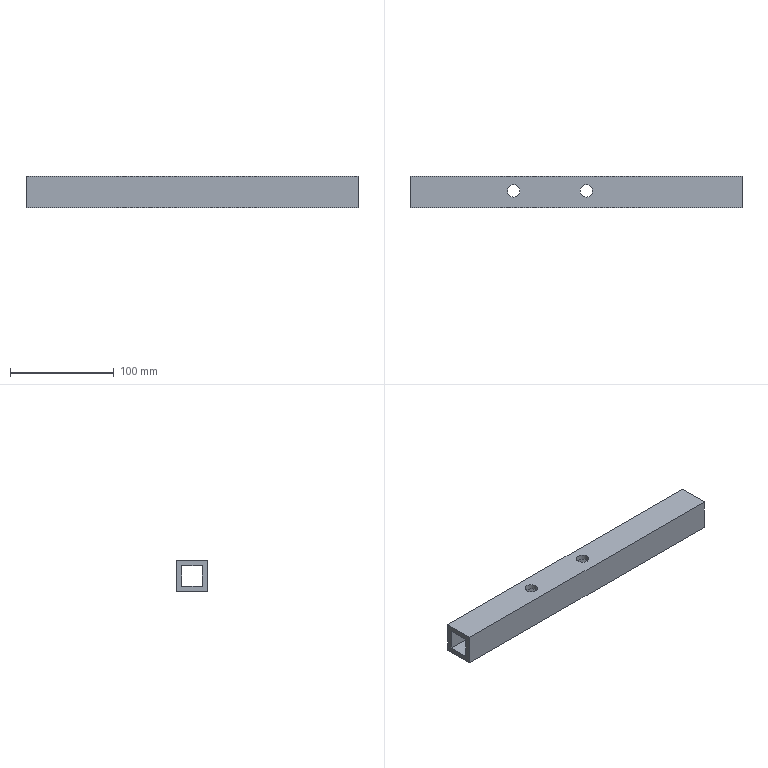Part | NX | features solid 2 | 1 solid | 14 faces | box 320 x 30 x 30 mm | volume 157738 mm3 | plane 10 | cylinder 4 | commonest cylinder face diameters 12 x4
STEP:
#1=CARTESIAN_POINT('',(65.,-206.,-122.));
#2=VERTEX_POINT('',#1);
#3=CARTESIAN_POINT('',(385.,-206.,-122.));
#4=VERTEX_POINT('',#3);
#5=CARTESIAN_POINT('',(132.005,-206.,-122.));
#6=DIRECTION('',(1.,0.,0.));
#7=VECTOR('',#6,1000.);
#8=LINE('',#5,#7);
#9=EDGE_CURVE('',#2,#4,#8,.T.);
#10=ORIENTED_EDGE('',*,*,#9,.T.);
#11=CARTESIAN_POINT('',(385.,-236.,-122.));
#12=VERTEX_POINT('',#11);
#13=CARTESIAN_POINT('',(385.,5.001,-122.));
#14=DIRECTION('',(0.,1.,0.));
#15=VECTOR('',#14,1000.);
#16=LINE('',#13,#15);
#17=EDGE_CURVE('',#12,#4,#16,.T.);
#18=ORIENTED_EDGE('',*,*,#17,.F.);
#19=CARTESIAN_POINT('',(65.,-236.,-122.));
#20=VERTEX_POINT('',#19);
#21=CARTESIAN_POINT('',(292.505,-236.,-122.));
#22=DIRECTION('',(1.,0.,0.));
#23=VECTOR('',#22,1000.);
#24=LINE('',#21,#23);
#25=EDGE_CURVE('',#20,#12,#24,.T.);
#26=ORIENTED_EDGE('',*,*,#25,.F.);
#27=CARTESIAN_POINT('',(65.,-206.,-122.));
#28=DIRECTION('',(0.,-1.,0.));
#29=VECTOR('',#28,1000.);
#30=LINE('',#27,#29);
#31=EDGE_CURVE('',#2,#20,#30,.T.);
#32=ORIENTED_EDGE('',*,*,#31,.F.);
#33=EDGE_LOOP('',(#10,#18,#26,#32));
#34=FACE_BOUND('',#33,.T.);
#35=CARTESIAN_POINT('',(165.,-226.,-122.));
#36=VERTEX_POINT('',#35);
#37=CARTESIAN_POINT('',(165.,-220.,-122.));
#38=DIRECTION('',(0.,0.,-1.));
#39=DIRECTION('',(0.,-1.,0.));
#40=AXIS2_PLACEMENT_3D('',#37,#38,#39);
#41=CIRCLE('',#40,6.);
#42=EDGE_CURVE('',#36,#36,#41,.T.);
#43=ORIENTED_EDGE('',*,*,#42,.F.);
#44=EDGE_LOOP('',(#43));
#45=FACE_BOUND('',#44,.T.);
#46=CARTESIAN_POINT('',(235.,-226.,-122.));
#47=VERTEX_POINT('',#46);
#48=CARTESIAN_POINT('',(235.,-220.,-122.));
#49=DIRECTION('',(0.,0.,1.));
#50=DIRECTION('',(0.,-1.,0.));
#51=AXIS2_PLACEMENT_3D('',#48,#49,#50);
#52=CIRCLE('',#51,6.);
#53=EDGE_CURVE('',#47,#47,#52,.T.);
#54=ORIENTED_EDGE('',*,*,#53,.T.);
#55=EDGE_LOOP('',(#54));
#56=FACE_BOUND('',#55,.T.);
#57=CARTESIAN_POINT('',(132.005,-206.5,-122.));
#58=DIRECTION('',(0.,0.,-1.));
#59=DIRECTION('',(0.,-1.,0.));
#60=AXIS2_PLACEMENT_3D('',#57,#58,#59);
#61=PLANE('',#60);
#62=ADVANCED_FACE('',(#34,#45,#56),#61,.T.);
#63=CARTESIAN_POINT('',(65.,-236.,-92.));
#64=VERTEX_POINT('',#63);
#65=CARTESIAN_POINT('',(385.,-236.,-92.));
#66=VERTEX_POINT('',#65);
#67=CARTESIAN_POINT('',(132.005,-236.,-92.));
#68=DIRECTION('',(1.,0.,0.));
#69=VECTOR('',#68,1000.);
#70=LINE('',#67,#69);
#71=EDGE_CURVE('',#64,#66,#70,.T.);
#72=ORIENTED_EDGE('',*,*,#71,.T.);
#73=CARTESIAN_POINT('',(385.,-206.,-92.));
#74=VERTEX_POINT('',#73);
#75=CARTESIAN_POINT('',(385.,5.001,-92.));
#76=DIRECTION('',(0.,-1.,0.));
#77=VECTOR('',#76,1000.);
#78=LINE('',#75,#77);
#79=EDGE_CURVE('',#74,#66,#78,.T.);
#80=ORIENTED_EDGE('',*,*,#79,.F.);
#81=CARTESIAN_POINT('',(65.,-206.,-92.));
#82=VERTEX_POINT('',#81);
#83=CARTESIAN_POINT('',(132.005,-206.,-92.));
#84=DIRECTION('',(1.,0.,0.));
#85=VECTOR('',#84,1000.);
#86=LINE('',#83,#85);
#87=EDGE_CURVE('',#82,#74,#86,.T.);
#88=ORIENTED_EDGE('',*,*,#87,.F.);
#89=CARTESIAN_POINT('',(65.,-236.5,-92.));
#90=DIRECTION('',(0.,1.,0.));
#91=VECTOR('',#90,1000.);
#92=LINE('',#89,#91);
#93=EDGE_CURVE('',#64,#82,#92,.T.);
#94=ORIENTED_EDGE('',*,*,#93,.F.);
#95=EDGE_LOOP('',(#72,#80,#88,#94));
#96=FACE_BOUND('',#95,.T.);
#97=CARTESIAN_POINT('',(165.,-226.,-92.));
#98=VERTEX_POINT('',#97);
#99=CARTESIAN_POINT('',(165.,-220.,-92.));
#100=DIRECTION('',(0.,0.,1.));
#101=DIRECTION('',(0.,-1.,0.));
#102=AXIS2_PLACEMENT_3D('',#99,#100,#101);
#103=CIRCLE('',#102,6.);
#104=EDGE_CURVE('',#98,#98,#103,.T.);
#105=ORIENTED_EDGE('',*,*,#104,.F.);
#106=EDGE_LOOP('',(#105));
#107=FACE_BOUND('',#106,.T.);
#108=CARTESIAN_POINT('',(235.,-226.,-92.));
#109=VERTEX_POINT('',#108);
#110=CARTESIAN_POINT('',(235.,-220.,-92.));
#111=DIRECTION('',(0.,0.,1.));
#112=DIRECTION('',(0.,-1.,0.));
#113=AXIS2_PLACEMENT_3D('',#110,#111,#112);
#114=CIRCLE('',#113,6.);
#115=EDGE_CURVE('',#109,#109,#114,.F.);
#116=ORIENTED_EDGE('',*,*,#115,.T.);
#117=EDGE_LOOP('',(#116));
#118=FACE_BOUND('',#117,.T.);
#119=CARTESIAN_POINT('',(132.005,-236.5,-92.));
#120=DIRECTION('',(0.,0.,1.));
#121=DIRECTION('',(0.,1.,0.));
#122=AXIS2_PLACEMENT_3D('',#119,#120,#121);
#123=PLANE('',#122);
#124=ADVANCED_FACE('',(#96,#107,#118),#123,.T.);
#125=CARTESIAN_POINT('',(65.,-211.,-117.));
#126=VERTEX_POINT('',#125);
#127=CARTESIAN_POINT('',(385.,-211.,-117.));
#128=VERTEX_POINT('',#127);
#129=CARTESIAN_POINT('',(132.005,-211.,-117.));
#130=DIRECTION('',(1.,0.,0.));
#131=VECTOR('',#130,1000.);
#132=LINE('',#129,#131);
#133=EDGE_CURVE('',#126,#128,#132,.T.);
#134=ORIENTED_EDGE('',*,*,#133,.F.);
#135=CARTESIAN_POINT('',(65.,-231.,-117.));
#136=VERTEX_POINT('',#135);
#137=CARTESIAN_POINT('',(65.,-206.5,-117.));
#138=DIRECTION('',(0.,-1.,0.));
#139=VECTOR('',#138,1000.);
#140=LINE('',#137,#139);
#141=EDGE_CURVE('',#126,#136,#140,.T.);
#142=ORIENTED_EDGE('',*,*,#141,.T.);
#143=CARTESIAN_POINT('',(385.,-231.,-117.));
#144=VERTEX_POINT('',#143);
#145=CARTESIAN_POINT('',(292.505,-231.,-117.));
#146=DIRECTION('',(1.,0.,0.));
#147=VECTOR('',#146,1000.);
#148=LINE('',#145,#147);
#149=EDGE_CURVE('',#136,#144,#148,.T.);
#150=ORIENTED_EDGE('',*,*,#149,.T.);
#151=CARTESIAN_POINT('',(385.,5.001,-117.));
#152=DIRECTION('',(0.,1.,0.));
#153=VECTOR('',#152,1000.);
#154=LINE('',#151,#153);
#155=EDGE_CURVE('',#144,#128,#154,.T.);
#156=ORIENTED_EDGE('',*,*,#155,.T.);
#157=EDGE_LOOP('',(#134,#142,#150,#156));
#158=FACE_BOUND('',#157,.T.);
#159=CARTESIAN_POINT('',(165.,-214.,-117.));
#160=VERTEX_POINT('',#159);
#161=CARTESIAN_POINT('',(165.,-220.,-117.));
#162=DIRECTION('',(0.,0.,-1.));
#163=DIRECTION('',(0.,1.,0.));
#164=AXIS2_PLACEMENT_3D('',#161,#162,#163);
#165=CIRCLE('',#164,6.);
#166=EDGE_CURVE('',#160,#160,#165,.T.);
#167=ORIENTED_EDGE('',*,*,#166,.T.);
#168=EDGE_LOOP('',(#167));
#169=FACE_BOUND('',#168,.T.);
#170=CARTESIAN_POINT('',(235.,-214.,-117.));
#171=VERTEX_POINT('',#170);
#172=CARTESIAN_POINT('',(235.,-220.,-117.));
#173=DIRECTION('',(0.,0.,-1.));
#174=DIRECTION('',(0.,1.,0.));
#175=AXIS2_PLACEMENT_3D('',#172,#173,#174);
#176=CIRCLE('',#175,6.);
#177=EDGE_CURVE('',#171,#171,#176,.F.);
#178=ORIENTED_EDGE('',*,*,#177,.F.);
#179=EDGE_LOOP('',(#178));
#180=FACE_BOUND('',#179,.T.);
#181=CARTESIAN_POINT('',(132.005,-206.5,-117.));
#182=DIRECTION('',(0.,0.,-1.));
#183=DIRECTION('',(0.,-1.,0.));
#184=AXIS2_PLACEMENT_3D('',#181,#182,#183);
#185=PLANE('',#184);
#186=ADVANCED_FACE('',(#158,#169,#180),#185,.F.);
#187=CARTESIAN_POINT('',(65.,-231.,-97.));
#188=VERTEX_POINT('',#187);
#189=CARTESIAN_POINT('',(385.,-231.,-97.));
#190=VERTEX_POINT('',#189);
#191=CARTESIAN_POINT('',(132.005,-231.,-97.));
#192=DIRECTION('',(1.,0.,0.));
#193=VECTOR('',#192,1000.);
#194=LINE('',#191,#193);
#195=EDGE_CURVE('',#188,#190,#194,.T.);
#196=ORIENTED_EDGE('',*,*,#195,.F.);
#197=CARTESIAN_POINT('',(65.,-211.,-97.));
#198=VERTEX_POINT('',#197);
#199=CARTESIAN_POINT('',(65.,-236.5,-97.));
#200=DIRECTION('',(0.,1.,0.));
#201=VECTOR('',#200,1000.);
#202=LINE('',#199,#201);
#203=EDGE_CURVE('',#188,#198,#202,.T.);
#204=ORIENTED_EDGE('',*,*,#203,.T.);
#205=CARTESIAN_POINT('',(385.,-211.,-97.));
#206=VERTEX_POINT('',#205);
#207=CARTESIAN_POINT('',(132.005,-211.,-97.));
#208=DIRECTION('',(1.,0.,0.));
#209=VECTOR('',#208,1000.);
#210=LINE('',#207,#209);
#211=EDGE_CURVE('',#198,#206,#210,.T.);
#212=ORIENTED_EDGE('',*,*,#211,.T.);
#213=CARTESIAN_POINT('',(385.,5.001,-97.));
#214=DIRECTION('',(0.,-1.,0.));
#215=VECTOR('',#214,1000.);
#216=LINE('',#213,#215);
#217=EDGE_CURVE('',#206,#190,#216,.T.);
#218=ORIENTED_EDGE('',*,*,#217,.T.);
#219=EDGE_LOOP('',(#196,#204,#212,#218));
#220=FACE_BOUND('',#219,.T.);
#221=CARTESIAN_POINT('',(165.,-226.,-97.));
#222=VERTEX_POINT('',#221);
#223=CARTESIAN_POINT('',(165.,-220.,-97.));
#224=DIRECTION('',(0.,0.,1.));
#225=DIRECTION('',(0.,-1.,0.));
#226=AXIS2_PLACEMENT_3D('',#223,#224,#225);
#227=CIRCLE('',#226,6.);
#228=EDGE_CURVE('',#222,#222,#227,.T.);
#229=ORIENTED_EDGE('',*,*,#228,.T.);
#230=EDGE_LOOP('',(#229));
#231=FACE_BOUND('',#230,.T.);
#232=CARTESIAN_POINT('',(235.,-226.,-97.));
#233=VERTEX_POINT('',#232);
#234=CARTESIAN_POINT('',(235.,-220.,-97.));
#235=DIRECTION('',(0.,0.,1.));
#236=DIRECTION('',(0.,-1.,0.));
#237=AXIS2_PLACEMENT_3D('',#234,#235,#236);
#238=CIRCLE('',#237,6.);
#239=EDGE_CURVE('',#233,#233,#238,.F.);
#240=ORIENTED_EDGE('',*,*,#239,.F.);
#241=EDGE_LOOP('',(#240));
#242=FACE_BOUND('',#241,.T.);
#243=CARTESIAN_POINT('',(132.005,-236.5,-97.));
#244=DIRECTION('',(0.,0.,1.));
#245=DIRECTION('',(0.,1.,0.));
#246=AXIS2_PLACEMENT_3D('',#243,#244,#245);
#247=PLANE('',#246);
#248=ADVANCED_FACE('',(#220,#231,#242),#247,.F.);
#249=CARTESIAN_POINT('',(65.,-236.,-126.));
#250=DIRECTION('',(0.,0.,1.));
#251=VECTOR('',#250,1000.);
#252=LINE('',#249,#251);
#253=EDGE_CURVE('',#20,#64,#252,.T.);
#254=ORIENTED_EDGE('',*,*,#253,.T.);
#255=ORIENTED_EDGE('',*,*,#93,.T.);
#256=CARTESIAN_POINT('',(65.,-206.,-96.));
#257=DIRECTION('',(0.,0.,-1.));
#258=VECTOR('',#257,1000.);
#259=LINE('',#256,#258);
#260=EDGE_CURVE('',#82,#2,#259,.T.);
#261=ORIENTED_EDGE('',*,*,#260,.T.);
#262=ORIENTED_EDGE('',*,*,#31,.T.);
#263=EDGE_LOOP('',(#254,#255,#261,#262));
#264=FACE_BOUND('',#263,.T.);
#265=CARTESIAN_POINT('',(65.,-231.,-126.));
#266=DIRECTION('',(0.,0.,1.));
#267=VECTOR('',#266,1000.);
#268=LINE('',#265,#267);
#269=EDGE_CURVE('',#136,#188,#268,.T.);
#270=ORIENTED_EDGE('',*,*,#269,.F.);
#271=ORIENTED_EDGE('',*,*,#141,.F.);
#272=CARTESIAN_POINT('',(65.,-211.,-96.));
#273=DIRECTION('',(0.,0.,-1.));
#274=VECTOR('',#273,1000.);
#275=LINE('',#272,#274);
#276=EDGE_CURVE('',#198,#126,#275,.T.);
#277=ORIENTED_EDGE('',*,*,#276,.F.);
#278=ORIENTED_EDGE('',*,*,#203,.F.);
#279=EDGE_LOOP('',(#270,#271,#277,#278));
#280=FACE_BOUND('',#279,.T.);
#281=CARTESIAN_POINT('',(65.,5.001,-101.38));
#282=DIRECTION('',(1.,0.,0.));
#283=DIRECTION('',(0.,0.,-1.));
#284=AXIS2_PLACEMENT_3D('',#281,#282,#283);
#285=PLANE('',#284);
#286=ADVANCED_FACE('',(#264,#280),#285,.F.);
#287=ORIENTED_EDGE('',*,*,#87,.T.);
#288=CARTESIAN_POINT('',(385.,-206.,-79.38));
#289=DIRECTION('',(0.,0.,1.));
#290=VECTOR('',#289,1000.);
#291=LINE('',#288,#290);
#292=EDGE_CURVE('',#4,#74,#291,.T.);
#293=ORIENTED_EDGE('',*,*,#292,.F.);
#294=ORIENTED_EDGE('',*,*,#9,.F.);
#295=ORIENTED_EDGE('',*,*,#260,.F.);
#296=EDGE_LOOP('',(#287,#293,#294,#295));
#297=FACE_BOUND('',#296,.T.);
#298=CARTESIAN_POINT('',(132.005,-206.,-96.));
#299=DIRECTION('',(0.,1.,0.));
#300=DIRECTION('',(0.,0.,-1.));
#301=AXIS2_PLACEMENT_3D('',#298,#299,#300);
#302=PLANE('',#301);
#303=ADVANCED_FACE('',(#297),#302,.T.);
#304=ORIENTED_EDGE('',*,*,#25,.T.);
#305=CARTESIAN_POINT('',(385.,-236.,-79.38));
#306=DIRECTION('',(0.,0.,-1.));
#307=VECTOR('',#306,1000.);
#308=LINE('',#305,#307);
#309=EDGE_CURVE('',#66,#12,#308,.T.);
#310=ORIENTED_EDGE('',*,*,#309,.F.);
#311=ORIENTED_EDGE('',*,*,#71,.F.);
#312=ORIENTED_EDGE('',*,*,#253,.F.);
#313=EDGE_LOOP('',(#304,#310,#311,#312));
#314=FACE_BOUND('',#313,.T.);
#315=CARTESIAN_POINT('',(292.505,-236.,-126.));
#316=DIRECTION('',(0.,-1.,0.));
#317=DIRECTION('',(0.,0.,1.));
#318=AXIS2_PLACEMENT_3D('',#315,#316,#317);
#319=PLANE('',#318);
#320=ADVANCED_FACE('',(#314),#319,.T.);
#321=CARTESIAN_POINT('',(385.,-231.,-79.38));
#322=DIRECTION('',(0.,0.,-1.));
#323=VECTOR('',#322,1000.);
#324=LINE('',#321,#323);
#325=EDGE_CURVE('',#190,#144,#324,.T.);
#326=ORIENTED_EDGE('',*,*,#325,.F.);
#327=ORIENTED_EDGE('',*,*,#217,.F.);
#328=CARTESIAN_POINT('',(385.,-211.,-79.38));
#329=DIRECTION('',(0.,0.,1.));
#330=VECTOR('',#329,1000.);
#331=LINE('',#328,#330);
#332=EDGE_CURVE('',#128,#206,#331,.T.);
#333=ORIENTED_EDGE('',*,*,#332,.F.);
#334=ORIENTED_EDGE('',*,*,#155,.F.);
#335=EDGE_LOOP('',(#326,#327,#333,#334));
#336=FACE_BOUND('',#335,.T.);
#337=ORIENTED_EDGE('',*,*,#309,.T.);
#338=ORIENTED_EDGE('',*,*,#17,.T.);
#339=ORIENTED_EDGE('',*,*,#292,.T.);
#340=ORIENTED_EDGE('',*,*,#79,.T.);
#341=EDGE_LOOP('',(#337,#338,#339,#340));
#342=FACE_BOUND('',#341,.T.);
#343=CARTESIAN_POINT('',(385.,5.001,-79.38));
#344=DIRECTION('',(1.,0.,0.));
#345=DIRECTION('',(0.,0.,1.));
#346=AXIS2_PLACEMENT_3D('',#343,#344,#345);
#347=PLANE('',#346);
#348=ADVANCED_FACE('',(#336,#342),#347,.T.);
#349=ORIENTED_EDGE('',*,*,#211,.F.);
#350=ORIENTED_EDGE('',*,*,#276,.T.);
#351=ORIENTED_EDGE('',*,*,#133,.T.);
#352=ORIENTED_EDGE('',*,*,#332,.T.);
#353=EDGE_LOOP('',(#349,#350,#351,#352));
#354=FACE_BOUND('',#353,.T.);
#355=CARTESIAN_POINT('',(132.005,-211.,-96.));
#356=DIRECTION('',(0.,1.,0.));
#357=DIRECTION('',(0.,0.,-1.));
#358=AXIS2_PLACEMENT_3D('',#355,#356,#357);
#359=PLANE('',#358);
#360=ADVANCED_FACE('',(#354),#359,.F.);
#361=ORIENTED_EDGE('',*,*,#149,.F.);
#362=ORIENTED_EDGE('',*,*,#269,.T.);
#363=ORIENTED_EDGE('',*,*,#195,.T.);
#364=ORIENTED_EDGE('',*,*,#325,.T.);
#365=EDGE_LOOP('',(#361,#362,#363,#364));
#366=FACE_BOUND('',#365,.T.);
#367=CARTESIAN_POINT('',(292.505,-231.,-126.));
#368=DIRECTION('',(0.,-1.,0.));
#369=DIRECTION('',(0.,0.,1.));
#370=AXIS2_PLACEMENT_3D('',#367,#368,#369);
#371=PLANE('',#370);
#372=ADVANCED_FACE('',(#366),#371,.F.);
#373=ORIENTED_EDGE('',*,*,#104,.T.);
#374=EDGE_LOOP('',(#373));
#375=FACE_BOUND('',#374,.T.);
#376=ORIENTED_EDGE('',*,*,#228,.F.);
#377=EDGE_LOOP('',(#376));
#378=FACE_BOUND('',#377,.T.);
#379=CARTESIAN_POINT('',(165.,-220.,-22.));
#380=DIRECTION('',(0.,0.,-1.));
#381=DIRECTION('',(-1.,0.,0.));
#382=AXIS2_PLACEMENT_3D('',#379,#380,#381);
#383=CYLINDRICAL_SURFACE('',#382,6.);
#384=ADVANCED_FACE('',(#375,#378),#383,.F.);
#385=ORIENTED_EDGE('',*,*,#42,.T.);
#386=EDGE_LOOP('',(#385));
#387=FACE_BOUND('',#386,.T.);
#388=ORIENTED_EDGE('',*,*,#166,.F.);
#389=EDGE_LOOP('',(#388));
#390=FACE_BOUND('',#389,.T.);
#391=CARTESIAN_POINT('',(165.,-220.,-22.));
#392=DIRECTION('',(0.,0.,-1.));
#393=DIRECTION('',(-1.,0.,0.));
#394=AXIS2_PLACEMENT_3D('',#391,#392,#393);
#395=CYLINDRICAL_SURFACE('',#394,6.);
#396=ADVANCED_FACE('',(#387,#390),#395,.F.);
#397=ORIENTED_EDGE('',*,*,#115,.F.);
#398=EDGE_LOOP('',(#397));
#399=FACE_BOUND('',#398,.T.);
#400=ORIENTED_EDGE('',*,*,#239,.T.);
#401=EDGE_LOOP('',(#400));
#402=FACE_BOUND('',#401,.T.);
#403=CARTESIAN_POINT('',(235.,-220.,-22.));
#404=DIRECTION('',(0.,0.,-1.));
#405=DIRECTION('',(-1.,0.,0.));
#406=AXIS2_PLACEMENT_3D('',#403,#404,#405);
#407=CYLINDRICAL_SURFACE('',#406,6.);
#408=ADVANCED_FACE('',(#399,#402),#407,.F.);
#409=ORIENTED_EDGE('',*,*,#53,.F.);
#410=EDGE_LOOP('',(#409));
#411=FACE_BOUND('',#410,.T.);
#412=ORIENTED_EDGE('',*,*,#177,.T.);
#413=EDGE_LOOP('',(#412));
#414=FACE_BOUND('',#413,.T.);
#415=CARTESIAN_POINT('',(235.,-220.,-22.));
#416=DIRECTION('',(0.,0.,-1.));
#417=DIRECTION('',(-1.,0.,0.));
#418=AXIS2_PLACEMENT_3D('',#415,#416,#417);
#419=CYLINDRICAL_SURFACE('',#418,6.);
#420=ADVANCED_FACE('',(#411,#414),#419,.F.);
#421=CLOSED_SHELL('',(#62,#124,#186,#248,#286,#303,#320,#348,#360,#372,#384,#396,#408,#420));
#422=MANIFOLD_SOLID_BREP('',#421);
#423=(LENGTH_UNIT()NAMED_UNIT(*)SI_UNIT(.MILLI.,.METRE.));
#424=UNCERTAINTY_MEASURE_WITH_UNIT(LENGTH_MEASURE(0.00001),#423,'','');
#425=(NAMED_UNIT(*)PLANE_ANGLE_UNIT()SI_UNIT($,.RADIAN.));
#426=(NAMED_UNIT(*)SI_UNIT($,.STERADIAN.)SOLID_ANGLE_UNIT());
#427=(GEOMETRIC_REPRESENTATION_CONTEXT(3)GLOBAL_UNCERTAINTY_ASSIGNED_CONTEXT((#424))GLOBAL_UNIT_ASSIGNED_CONTEXT((#423,#425,#426))REPRESENTATION_CONTEXT('',''));
#428=ADVANCED_BREP_SHAPE_REPRESENTATION('',(#422),#427);